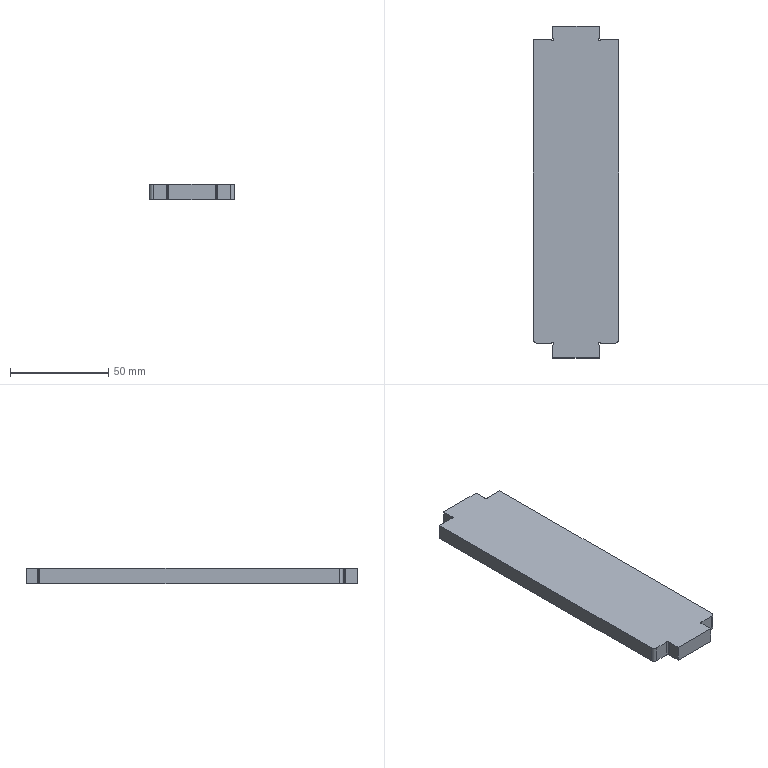Part | SolidWorks | features Fillet 2, FlatPattern 1, ICE 1, SMBaseFlange 1, SheetMetal 1 | 1 solid | 30 faces | box 43.5 x 169.3 x 8 mm | volume 56573 mm3 | cylinder 16 | plane 14 | commonest cylinder face diameters 2 x8 1 x6 4 x2
STEP:
#1=CARTESIAN_POINT('',(-156.793,-408.685,0.));
#2=VERTEX_POINT('',#1);
#3=CARTESIAN_POINT('',(-157.569,-409.102,0.));
#4=VERTEX_POINT('',#3);
#5=CARTESIAN_POINT('',(-157.069,-409.102,0.));
#6=DIRECTION('',(0.,0.,1.));
#7=DIRECTION('',(1.,0.,0.));
#8=AXIS2_PLACEMENT_3D('',#5,#6,#7);
#9=CIRCLE('',#8,0.5);
#10=EDGE_CURVE('',#2,#4,#9,.T.);
#11=ORIENTED_EDGE('',*,*,#10,.T.);
#12=CARTESIAN_POINT('',(-157.569,-409.102,-8.));
#13=VERTEX_POINT('',#12);
#14=CARTESIAN_POINT('',(-157.569,-409.102,-8.));
#15=DIRECTION('',(0.,0.,-1.));
#16=VECTOR('',#15,1000.);
#17=LINE('',#14,#16);
#18=EDGE_CURVE('',#4,#13,#17,.T.);
#19=ORIENTED_EDGE('',*,*,#18,.T.);
#20=CARTESIAN_POINT('',(-156.793,-408.685,-8.));
#21=VERTEX_POINT('',#20);
#22=CARTESIAN_POINT('',(-157.069,-409.102,-8.));
#23=DIRECTION('',(0.,0.,1.));
#24=DIRECTION('',(1.,0.,0.));
#25=AXIS2_PLACEMENT_3D('',#22,#23,#24);
#26=CIRCLE('',#25,0.5);
#27=EDGE_CURVE('',#21,#13,#26,.T.);
#28=ORIENTED_EDGE('',*,*,#27,.F.);
#29=CARTESIAN_POINT('',(-156.793,-408.685,-8.));
#30=DIRECTION('',(0.,0.,1.));
#31=VECTOR('',#30,1000.);
#32=LINE('',#29,#31);
#33=EDGE_CURVE('',#21,#2,#32,.T.);
#34=ORIENTED_EDGE('',*,*,#33,.T.);
#35=EDGE_LOOP('',(#11,#19,#28,#34));
#36=FACE_OUTER_BOUND('',#35,.T.);
#37=CARTESIAN_POINT('',(-157.069,-409.102,-8.));
#38=DIRECTION('',(0.,0.,-1.));
#39=DIRECTION('',(-1.,0.,0.));
#40=AXIS2_PLACEMENT_3D('',#37,#38,#39);
#41=CYLINDRICAL_SURFACE('',#40,0.5);
#42=ADVANCED_FACE('',(#36),#41,.F.);
#43=CARTESIAN_POINT('',(-157.486,-253.526,0.));
#44=VERTEX_POINT('',#43);
#45=CARTESIAN_POINT('',(-157.569,-253.802,0.));
#46=VERTEX_POINT('',#45);
#47=CARTESIAN_POINT('',(-157.069,-253.802,0.));
#48=DIRECTION('',(0.,0.,1.));
#49=DIRECTION('',(1.,0.,0.));
#50=AXIS2_PLACEMENT_3D('',#47,#48,#49);
#51=CIRCLE('',#50,0.5);
#52=EDGE_CURVE('',#44,#46,#51,.T.);
#53=ORIENTED_EDGE('',*,*,#52,.T.);
#54=CARTESIAN_POINT('',(-157.569,-253.802,-8.));
#55=VERTEX_POINT('',#54);
#56=CARTESIAN_POINT('',(-157.569,-253.802,-8.));
#57=DIRECTION('',(0.,0.,-1.));
#58=VECTOR('',#57,1000.);
#59=LINE('',#56,#58);
#60=EDGE_CURVE('',#46,#55,#59,.T.);
#61=ORIENTED_EDGE('',*,*,#60,.T.);
#62=CARTESIAN_POINT('',(-157.486,-253.526,-8.));
#63=VERTEX_POINT('',#62);
#64=CARTESIAN_POINT('',(-157.069,-253.802,-8.));
#65=DIRECTION('',(0.,0.,1.));
#66=DIRECTION('',(1.,0.,0.));
#67=AXIS2_PLACEMENT_3D('',#64,#65,#66);
#68=CIRCLE('',#67,0.5);
#69=EDGE_CURVE('',#63,#55,#68,.T.);
#70=ORIENTED_EDGE('',*,*,#69,.F.);
#71=CARTESIAN_POINT('',(-157.486,-253.526,-8.));
#72=DIRECTION('',(0.,0.,1.));
#73=VECTOR('',#72,1000.);
#74=LINE('',#71,#73);
#75=EDGE_CURVE('',#63,#44,#74,.T.);
#76=ORIENTED_EDGE('',*,*,#75,.T.);
#77=EDGE_LOOP('',(#53,#61,#70,#76));
#78=FACE_OUTER_BOUND('',#77,.T.);
#79=CARTESIAN_POINT('',(-157.069,-253.802,-8.));
#80=DIRECTION('',(0.,0.,-1.));
#81=DIRECTION('',(-1.,0.,0.));
#82=AXIS2_PLACEMENT_3D('',#79,#80,#81);
#83=CYLINDRICAL_SURFACE('',#82,0.5);
#84=ADVANCED_FACE('',(#78),#83,.F.);
#85=CARTESIAN_POINT('',(-188.819,-408.852,0.));
#86=VERTEX_POINT('',#85);
#87=CARTESIAN_POINT('',(-181.898,-408.852,0.));
#88=VERTEX_POINT('',#87);
#89=CARTESIAN_POINT('',(-180.819,-408.852,0.));
#90=DIRECTION('',(1.,0.,0.));
#91=VECTOR('',#90,1000.);
#92=LINE('',#89,#91);
#93=EDGE_CURVE('',#86,#88,#92,.T.);
#94=ORIENTED_EDGE('',*,*,#93,.F.);
#95=CARTESIAN_POINT('',(-188.819,-408.852,-8.));
#96=VERTEX_POINT('',#95);
#97=CARTESIAN_POINT('',(-188.819,-408.852,-8.));
#98=DIRECTION('',(0.,0.,-1.));
#99=VECTOR('',#98,1000.);
#100=LINE('',#97,#99);
#101=EDGE_CURVE('',#86,#96,#100,.T.);
#102=ORIENTED_EDGE('',*,*,#101,.T.);
#103=CARTESIAN_POINT('',(-181.898,-408.852,-8.));
#104=VERTEX_POINT('',#103);
#105=CARTESIAN_POINT('',(-180.819,-408.852,-8.));
#106=DIRECTION('',(1.,0.,0.));
#107=VECTOR('',#106,1000.);
#108=LINE('',#105,#107);
#109=EDGE_CURVE('',#96,#104,#108,.T.);
#110=ORIENTED_EDGE('',*,*,#109,.T.);
#111=CARTESIAN_POINT('',(-181.898,-408.852,-8.));
#112=DIRECTION('',(0.,0.,1.));
#113=VECTOR('',#112,1000.);
#114=LINE('',#111,#113);
#115=EDGE_CURVE('',#104,#88,#114,.T.);
#116=ORIENTED_EDGE('',*,*,#115,.T.);
#117=EDGE_LOOP('',(#94,#102,#110,#116));
#118=FACE_OUTER_BOUND('',#117,.T.);
#119=CARTESIAN_POINT('',(-180.819,-408.852,-8.));
#120=DIRECTION('',(0.,-1.,0.));
#121=DIRECTION('',(0.,0.,-1.));
#122=AXIS2_PLACEMENT_3D('',#119,#120,#121);
#123=PLANE('',#122);
#124=ADVANCED_FACE('',(#118),#123,.T.);
#125=CARTESIAN_POINT('',(-181.898,-254.052,0.));
#126=VERTEX_POINT('',#125);
#127=CARTESIAN_POINT('',(-190.819,-254.052,0.));
#128=VERTEX_POINT('',#127);
#129=CARTESIAN_POINT('',(-190.819,-254.052,0.));
#130=DIRECTION('',(-1.,0.,0.));
#131=VECTOR('',#130,1000.);
#132=LINE('',#129,#131);
#133=EDGE_CURVE('',#126,#128,#132,.T.);
#134=ORIENTED_EDGE('',*,*,#133,.F.);
#135=CARTESIAN_POINT('',(-181.898,-254.052,-8.));
#136=VERTEX_POINT('',#135);
#137=CARTESIAN_POINT('',(-181.898,-254.052,-8.));
#138=DIRECTION('',(0.,0.,-1.));
#139=VECTOR('',#138,1000.);
#140=LINE('',#137,#139);
#141=EDGE_CURVE('',#126,#136,#140,.T.);
#142=ORIENTED_EDGE('',*,*,#141,.T.);
#143=CARTESIAN_POINT('',(-190.819,-254.052,-8.));
#144=VERTEX_POINT('',#143);
#145=CARTESIAN_POINT('',(-190.819,-254.052,-8.));
#146=DIRECTION('',(-1.,0.,0.));
#147=VECTOR('',#146,1000.);
#148=LINE('',#145,#147);
#149=EDGE_CURVE('',#136,#144,#148,.T.);
#150=ORIENTED_EDGE('',*,*,#149,.T.);
#151=CARTESIAN_POINT('',(-190.819,-254.052,-8.));
#152=DIRECTION('',(0.,0.,1.));
#153=VECTOR('',#152,1000.);
#154=LINE('',#151,#153);
#155=EDGE_CURVE('',#144,#128,#154,.T.);
#156=ORIENTED_EDGE('',*,*,#155,.T.);
#157=EDGE_LOOP('',(#134,#142,#150,#156));
#158=FACE_OUTER_BOUND('',#157,.T.);
#159=CARTESIAN_POINT('',(-190.819,-254.052,-8.));
#160=DIRECTION('',(0.,1.,0.));
#161=DIRECTION('',(-1.,0.,0.));
#162=AXIS2_PLACEMENT_3D('',#159,#160,#161);
#163=PLANE('',#162);
#164=ADVANCED_FACE('',(#158),#163,.T.);
#165=CARTESIAN_POINT('',(-180.819,-247.052,-8.));
#166=VERTEX_POINT('',#165);
#167=CARTESIAN_POINT('',(-180.819,-252.973,-8.));
#168=VERTEX_POINT('',#167);
#169=CARTESIAN_POINT('',(-180.819,-247.052,-8.));
#170=DIRECTION('',(0.,-1.,0.));
#171=VECTOR('',#170,1000.);
#172=LINE('',#169,#171);
#173=EDGE_CURVE('',#166,#168,#172,.T.);
#174=ORIENTED_EDGE('',*,*,#173,.T.);
#175=CARTESIAN_POINT('',(-180.819,-252.973,0.));
#176=VERTEX_POINT('',#175);
#177=CARTESIAN_POINT('',(-180.819,-252.973,-8.));
#178=DIRECTION('',(0.,0.,1.));
#179=VECTOR('',#178,1000.);
#180=LINE('',#177,#179);
#181=EDGE_CURVE('',#168,#176,#180,.T.);
#182=ORIENTED_EDGE('',*,*,#181,.T.);
#183=CARTESIAN_POINT('',(-180.819,-247.052,0.));
#184=VERTEX_POINT('',#183);
#185=CARTESIAN_POINT('',(-180.819,-247.052,0.));
#186=DIRECTION('',(0.,-1.,0.));
#187=VECTOR('',#186,1000.);
#188=LINE('',#185,#187);
#189=EDGE_CURVE('',#184,#176,#188,.T.);
#190=ORIENTED_EDGE('',*,*,#189,.F.);
#191=CARTESIAN_POINT('',(-180.819,-247.052,-8.));
#192=DIRECTION('',(0.,0.,1.));
#193=VECTOR('',#192,1000.);
#194=LINE('',#191,#193);
#195=EDGE_CURVE('',#166,#184,#194,.T.);
#196=ORIENTED_EDGE('',*,*,#195,.F.);
#197=EDGE_LOOP('',(#174,#182,#190,#196));
#198=FACE_OUTER_BOUND('',#197,.T.);
#199=CARTESIAN_POINT('',(-180.819,-247.052,-8.));
#200=DIRECTION('',(-1.,0.,0.));
#201=DIRECTION('',(0.,-1.,0.));
#202=AXIS2_PLACEMENT_3D('',#199,#200,#201);
#203=PLANE('',#202);
#204=ADVANCED_FACE('',(#198),#203,.T.);
#205=CARTESIAN_POINT('',(-157.319,-252.973,0.));
#206=VERTEX_POINT('',#205);
#207=CARTESIAN_POINT('',(-157.319,-247.052,0.));
#208=VERTEX_POINT('',#207);
#209=CARTESIAN_POINT('',(-157.319,-254.052,0.));
#210=DIRECTION('',(0.,1.,0.));
#211=VECTOR('',#210,1000.);
#212=LINE('',#209,#211);
#213=EDGE_CURVE('',#206,#208,#212,.T.);
#214=ORIENTED_EDGE('',*,*,#213,.F.);
#215=CARTESIAN_POINT('',(-157.319,-252.973,-8.));
#216=VERTEX_POINT('',#215);
#217=CARTESIAN_POINT('',(-157.319,-252.973,-8.));
#218=DIRECTION('',(0.,0.,-1.));
#219=VECTOR('',#218,1000.);
#220=LINE('',#217,#219);
#221=EDGE_CURVE('',#206,#216,#220,.T.);
#222=ORIENTED_EDGE('',*,*,#221,.T.);
#223=CARTESIAN_POINT('',(-157.319,-247.052,-8.));
#224=VERTEX_POINT('',#223);
#225=CARTESIAN_POINT('',(-157.319,-254.052,-8.));
#226=DIRECTION('',(0.,1.,0.));
#227=VECTOR('',#226,1000.);
#228=LINE('',#225,#227);
#229=EDGE_CURVE('',#216,#224,#228,.T.);
#230=ORIENTED_EDGE('',*,*,#229,.T.);
#231=CARTESIAN_POINT('',(-157.319,-247.052,-8.));
#232=DIRECTION('',(0.,0.,1.));
#233=VECTOR('',#232,1000.);
#234=LINE('',#231,#233);
#235=EDGE_CURVE('',#224,#208,#234,.T.);
#236=ORIENTED_EDGE('',*,*,#235,.T.);
#237=EDGE_LOOP('',(#214,#222,#230,#236));
#238=FACE_OUTER_BOUND('',#237,.T.);
#239=CARTESIAN_POINT('',(-157.319,-254.052,-8.));
#240=DIRECTION('',(1.,0.,0.));
#241=DIRECTION('',(0.,1.,0.));
#242=AXIS2_PLACEMENT_3D('',#239,#240,#241);
#243=PLANE('',#242);
#244=ADVANCED_FACE('',(#238),#243,.T.);
#245=CARTESIAN_POINT('',(-147.319,-254.052,-8.));
#246=VERTEX_POINT('',#245);
#247=CARTESIAN_POINT('',(-156.24,-254.052,-8.));
#248=VERTEX_POINT('',#247);
#249=CARTESIAN_POINT('',(-157.319,-254.052,-8.));
#250=DIRECTION('',(-1.,0.,0.));
#251=VECTOR('',#250,1000.);
#252=LINE('',#249,#251);
#253=EDGE_CURVE('',#246,#248,#252,.T.);
#254=ORIENTED_EDGE('',*,*,#253,.T.);
#255=CARTESIAN_POINT('',(-156.24,-254.052,0.));
#256=VERTEX_POINT('',#255);
#257=CARTESIAN_POINT('',(-156.24,-254.052,-8.));
#258=DIRECTION('',(0.,0.,1.));
#259=VECTOR('',#258,1000.);
#260=LINE('',#257,#259);
#261=EDGE_CURVE('',#248,#256,#260,.T.);
#262=ORIENTED_EDGE('',*,*,#261,.T.);
#263=CARTESIAN_POINT('',(-147.319,-254.052,0.));
#264=VERTEX_POINT('',#263);
#265=CARTESIAN_POINT('',(-157.319,-254.052,0.));
#266=DIRECTION('',(-1.,0.,0.));
#267=VECTOR('',#266,1000.);
#268=LINE('',#265,#267);
#269=EDGE_CURVE('',#264,#256,#268,.T.);
#270=ORIENTED_EDGE('',*,*,#269,.F.);
#271=CARTESIAN_POINT('',(-147.319,-254.052,-8.));
#272=DIRECTION('',(0.,0.,1.));
#273=VECTOR('',#272,1000.);
#274=LINE('',#271,#273);
#275=EDGE_CURVE('',#246,#264,#274,.T.);
#276=ORIENTED_EDGE('',*,*,#275,.F.);
#277=EDGE_LOOP('',(#254,#262,#270,#276));
#278=FACE_OUTER_BOUND('',#277,.T.);
#279=CARTESIAN_POINT('',(-157.319,-254.052,-8.));
#280=DIRECTION('',(0.,1.,0.));
#281=DIRECTION('',(-1.,0.,0.));
#282=AXIS2_PLACEMENT_3D('',#279,#280,#281);
#283=PLANE('',#282);
#284=ADVANCED_FACE('',(#278),#283,.T.);
#285=CARTESIAN_POINT('',(-156.24,-408.852,-8.));
#286=VERTEX_POINT('',#285);
#287=CARTESIAN_POINT('',(-149.319,-408.852,-8.));
#288=VERTEX_POINT('',#287);
#289=CARTESIAN_POINT('',(-147.319,-408.852,-8.));
#290=DIRECTION('',(1.,0.,0.));
#291=VECTOR('',#290,1000.);
#292=LINE('',#289,#291);
#293=EDGE_CURVE('',#286,#288,#292,.T.);
#294=ORIENTED_EDGE('',*,*,#293,.T.);
#295=CARTESIAN_POINT('',(-149.319,-408.852,0.));
#296=VERTEX_POINT('',#295);
#297=CARTESIAN_POINT('',(-149.319,-408.852,-8.));
#298=DIRECTION('',(0.,0.,1.));
#299=VECTOR('',#298,1000.);
#300=LINE('',#297,#299);
#301=EDGE_CURVE('',#288,#296,#300,.T.);
#302=ORIENTED_EDGE('',*,*,#301,.T.);
#303=CARTESIAN_POINT('',(-156.24,-408.852,0.));
#304=VERTEX_POINT('',#303);
#305=CARTESIAN_POINT('',(-147.319,-408.852,0.));
#306=DIRECTION('',(1.,0.,0.));
#307=VECTOR('',#306,1000.);
#308=LINE('',#305,#307);
#309=EDGE_CURVE('',#304,#296,#308,.T.);
#310=ORIENTED_EDGE('',*,*,#309,.F.);
#311=CARTESIAN_POINT('',(-156.24,-408.852,-8.));
#312=DIRECTION('',(0.,0.,-1.));
#313=VECTOR('',#312,1000.);
#314=LINE('',#311,#313);
#315=EDGE_CURVE('',#304,#286,#314,.T.);
#316=ORIENTED_EDGE('',*,*,#315,.T.);
#317=EDGE_LOOP('',(#294,#302,#310,#316));
#318=FACE_OUTER_BOUND('',#317,.T.);
#319=CARTESIAN_POINT('',(-147.319,-408.852,-8.));
#320=DIRECTION('',(0.,-1.,0.));
#321=DIRECTION('',(1.,0.,0.));
#322=AXIS2_PLACEMENT_3D('',#319,#320,#321);
#323=PLANE('',#322);
#324=ADVANCED_FACE('',(#318),#323,.T.);
#325=CARTESIAN_POINT('',(-157.319,-416.352,-8.));
#326=VERTEX_POINT('',#325);
#327=CARTESIAN_POINT('',(-157.319,-409.931,-8.));
#328=VERTEX_POINT('',#327);
#329=CARTESIAN_POINT('',(-157.319,-408.852,-8.));
#330=DIRECTION('',(0.,1.,0.));
#331=VECTOR('',#330,1000.);
#332=LINE('',#329,#331);
#333=EDGE_CURVE('',#326,#328,#332,.T.);
#334=ORIENTED_EDGE('',*,*,#333,.T.);
#335=CARTESIAN_POINT('',(-157.319,-409.931,0.));
#336=VERTEX_POINT('',#335);
#337=CARTESIAN_POINT('',(-157.319,-409.931,-8.));
#338=DIRECTION('',(0.,0.,1.));
#339=VECTOR('',#338,1000.);
#340=LINE('',#337,#339);
#341=EDGE_CURVE('',#328,#336,#340,.T.);
#342=ORIENTED_EDGE('',*,*,#341,.T.);
#343=CARTESIAN_POINT('',(-157.319,-416.352,0.));
#344=VERTEX_POINT('',#343);
#345=CARTESIAN_POINT('',(-157.319,-408.852,0.));
#346=DIRECTION('',(0.,1.,0.));
#347=VECTOR('',#346,1000.);
#348=LINE('',#345,#347);
#349=EDGE_CURVE('',#344,#336,#348,.T.);
#350=ORIENTED_EDGE('',*,*,#349,.F.);
#351=CARTESIAN_POINT('',(-157.319,-416.352,-8.));
#352=DIRECTION('',(0.,0.,1.));
#353=VECTOR('',#352,1000.);
#354=LINE('',#351,#353);
#355=EDGE_CURVE('',#326,#344,#354,.T.);
#356=ORIENTED_EDGE('',*,*,#355,.F.);
#357=EDGE_LOOP('',(#334,#342,#350,#356));
#358=FACE_OUTER_BOUND('',#357,.T.);
#359=CARTESIAN_POINT('',(-157.319,-408.852,-8.));
#360=DIRECTION('',(1.,0.,0.));
#361=DIRECTION('',(0.,0.,-1.));
#362=AXIS2_PLACEMENT_3D('',#359,#360,#361);
#363=PLANE('',#362);
#364=ADVANCED_FACE('',(#358),#363,.T.);
#365=CARTESIAN_POINT('',(-180.819,-409.931,0.));
#366=VERTEX_POINT('',#365);
#367=CARTESIAN_POINT('',(-180.819,-416.352,0.));
#368=VERTEX_POINT('',#367);
#369=CARTESIAN_POINT('',(-180.819,-416.352,0.));
#370=DIRECTION('',(0.,-1.,0.));
#371=VECTOR('',#370,1000.);
#372=LINE('',#369,#371);
#373=EDGE_CURVE('',#366,#368,#372,.T.);
#374=ORIENTED_EDGE('',*,*,#373,.F.);
#375=CARTESIAN_POINT('',(-180.819,-409.931,-8.));
#376=VERTEX_POINT('',#375);
#377=CARTESIAN_POINT('',(-180.819,-409.931,-8.));
#378=DIRECTION('',(0.,0.,-1.));
#379=VECTOR('',#378,1000.);
#380=LINE('',#377,#379);
#381=EDGE_CURVE('',#366,#376,#380,.T.);
#382=ORIENTED_EDGE('',*,*,#381,.T.);
#383=CARTESIAN_POINT('',(-180.819,-416.352,-8.));
#384=VERTEX_POINT('',#383);
#385=CARTESIAN_POINT('',(-180.819,-416.352,-8.));
#386=DIRECTION('',(0.,-1.,0.));
#387=VECTOR('',#386,1000.);
#388=LINE('',#385,#387);
#389=EDGE_CURVE('',#376,#384,#388,.T.);
#390=ORIENTED_EDGE('',*,*,#389,.T.);
#391=CARTESIAN_POINT('',(-180.819,-416.352,-8.));
#392=DIRECTION('',(0.,0.,1.));
#393=VECTOR('',#392,1000.);
#394=LINE('',#391,#393);
#395=EDGE_CURVE('',#384,#368,#394,.T.);
#396=ORIENTED_EDGE('',*,*,#395,.T.);
#397=EDGE_LOOP('',(#374,#382,#390,#396));
#398=FACE_OUTER_BOUND('',#397,.T.);
#399=CARTESIAN_POINT('',(-180.819,-416.352,-8.));
#400=DIRECTION('',(-1.,0.,0.));
#401=DIRECTION('',(0.,-1.,0.));
#402=AXIS2_PLACEMENT_3D('',#399,#400,#401);
#403=PLANE('',#402);
#404=ADVANCED_FACE('',(#398),#403,.T.);
#405=ORIENTED_EDGE('',*,*,#109,.F.);
#406=CARTESIAN_POINT('',(-190.819,-406.852,-8.));
#407=VERTEX_POINT('',#406);
#408=CARTESIAN_POINT('',(-188.819,-406.852,-8.));
#409=DIRECTION('',(0.,0.,-1.));
#410=DIRECTION('',(-1.,0.,0.));
#411=AXIS2_PLACEMENT_3D('',#408,#409,#410);
#412=CIRCLE('',#411,2.);
#413=EDGE_CURVE('',#96,#407,#412,.T.);
#414=ORIENTED_EDGE('',*,*,#413,.T.);
#415=CARTESIAN_POINT('',(-190.819,-408.852,-8.));
#416=DIRECTION('',(0.,-1.,0.));
#417=VECTOR('',#416,1000.);
#418=LINE('',#415,#417);
#419=EDGE_CURVE('',#144,#407,#418,.T.);
#420=ORIENTED_EDGE('',*,*,#419,.F.);
#421=ORIENTED_EDGE('',*,*,#149,.F.);
#422=CARTESIAN_POINT('',(-181.346,-254.219,-8.));
#423=VERTEX_POINT('',#422);
#424=CARTESIAN_POINT('',(-181.898,-255.052,-8.));
#425=DIRECTION('',(0.,0.,-1.));
#426=DIRECTION('',(-1.,0.,0.));
#427=AXIS2_PLACEMENT_3D('',#424,#425,#426);
#428=CIRCLE('',#427,1.);
#429=EDGE_CURVE('',#136,#423,#428,.T.);
#430=ORIENTED_EDGE('',*,*,#429,.T.);
#431=CARTESIAN_POINT('',(-180.653,-253.526,-8.));
#432=VERTEX_POINT('',#431);
#433=CARTESIAN_POINT('',(-181.069,-253.802,-8.));
#434=DIRECTION('',(0.,0.,1.));
#435=DIRECTION('',(1.,0.,0.));
#436=AXIS2_PLACEMENT_3D('',#433,#434,#435);
#437=CIRCLE('',#436,0.5);
#438=EDGE_CURVE('',#423,#432,#437,.T.);
#439=ORIENTED_EDGE('',*,*,#438,.T.);
#440=CARTESIAN_POINT('',(-179.819,-252.973,-8.));
#441=DIRECTION('',(0.,0.,-1.));
#442=DIRECTION('',(-1.,0.,0.));
#443=AXIS2_PLACEMENT_3D('',#440,#441,#442);
#444=CIRCLE('',#443,1.);
#445=EDGE_CURVE('',#432,#168,#444,.T.);
#446=ORIENTED_EDGE('',*,*,#445,.T.);
#447=ORIENTED_EDGE('',*,*,#173,.F.);
#448=CARTESIAN_POINT('',(-157.319,-247.052,-8.));
#449=DIRECTION('',(-1.,0.,0.));
#450=VECTOR('',#449,1000.);
#451=LINE('',#448,#450);
#452=EDGE_CURVE('',#224,#166,#451,.T.);
#453=ORIENTED_EDGE('',*,*,#452,.F.);
#454=ORIENTED_EDGE('',*,*,#229,.F.);
#455=CARTESIAN_POINT('',(-158.319,-252.973,-8.));
#456=DIRECTION('',(0.,0.,-1.));
#457=DIRECTION('',(-1.,0.,0.));
#458=AXIS2_PLACEMENT_3D('',#455,#456,#457);
#459=CIRCLE('',#458,1.);
#460=EDGE_CURVE('',#216,#63,#459,.T.);
#461=ORIENTED_EDGE('',*,*,#460,.T.);
#462=ORIENTED_EDGE('',*,*,#69,.T.);
#463=CARTESIAN_POINT('',(-156.793,-254.219,-8.));
#464=VERTEX_POINT('',#463);
#465=CARTESIAN_POINT('',(-157.069,-253.802,-8.));
#466=DIRECTION('',(0.,0.,1.));
#467=DIRECTION('',(1.,0.,0.));
#468=AXIS2_PLACEMENT_3D('',#465,#466,#467);
#469=CIRCLE('',#468,0.5);
#470=EDGE_CURVE('',#55,#464,#469,.T.);
#471=ORIENTED_EDGE('',*,*,#470,.T.);
#472=CARTESIAN_POINT('',(-156.24,-255.052,-8.));
#473=DIRECTION('',(0.,0.,-1.));
#474=DIRECTION('',(-1.,0.,0.));
#475=AXIS2_PLACEMENT_3D('',#472,#473,#474);
#476=CIRCLE('',#475,1.);
#477=EDGE_CURVE('',#464,#248,#476,.T.);
#478=ORIENTED_EDGE('',*,*,#477,.T.);
#479=ORIENTED_EDGE('',*,*,#253,.F.);
#480=CARTESIAN_POINT('',(-147.319,-406.852,-8.));
#481=VERTEX_POINT('',#480);
#482=CARTESIAN_POINT('',(-147.319,-254.052,-8.));
#483=DIRECTION('',(0.,1.,0.));
#484=VECTOR('',#483,1000.);
#485=LINE('',#482,#484);
#486=EDGE_CURVE('',#481,#246,#485,.T.);
#487=ORIENTED_EDGE('',*,*,#486,.F.);
#488=CARTESIAN_POINT('',(-149.319,-406.852,-8.));
#489=DIRECTION('',(0.,0.,-1.));
#490=DIRECTION('',(-1.,0.,0.));
#491=AXIS2_PLACEMENT_3D('',#488,#489,#490);
#492=CIRCLE('',#491,2.);
#493=EDGE_CURVE('',#481,#288,#492,.T.);
#494=ORIENTED_EDGE('',*,*,#493,.T.);
#495=ORIENTED_EDGE('',*,*,#293,.F.);
#496=CARTESIAN_POINT('',(-156.24,-407.852,-8.));
#497=DIRECTION('',(0.,0.,-1.));
#498=DIRECTION('',(-1.,0.,0.));
#499=AXIS2_PLACEMENT_3D('',#496,#497,#498);
#500=CIRCLE('',#499,1.);
#501=EDGE_CURVE('',#286,#21,#500,.T.);
#502=ORIENTED_EDGE('',*,*,#501,.T.);
#503=ORIENTED_EDGE('',*,*,#27,.T.);
#504=CARTESIAN_POINT('',(-157.486,-409.378,-8.));
#505=VERTEX_POINT('',#504);
#506=CARTESIAN_POINT('',(-157.069,-409.102,-8.));
#507=DIRECTION('',(0.,0.,1.));
#508=DIRECTION('',(1.,0.,0.));
#509=AXIS2_PLACEMENT_3D('',#506,#507,#508);
#510=CIRCLE('',#509,0.5);
#511=EDGE_CURVE('',#13,#505,#510,.T.);
#512=ORIENTED_EDGE('',*,*,#511,.T.);
#513=CARTESIAN_POINT('',(-158.319,-409.931,-8.));
#514=DIRECTION('',(0.,0.,-1.));
#515=DIRECTION('',(-1.,0.,0.));
#516=AXIS2_PLACEMENT_3D('',#513,#514,#515);
#517=CIRCLE('',#516,1.);
#518=EDGE_CURVE('',#505,#328,#517,.T.);
#519=ORIENTED_EDGE('',*,*,#518,.T.);
#520=ORIENTED_EDGE('',*,*,#333,.F.);
#521=CARTESIAN_POINT('',(-157.319,-416.352,-8.));
#522=DIRECTION('',(1.,0.,0.));
#523=VECTOR('',#522,1000.);
#524=LINE('',#521,#523);
#525=EDGE_CURVE('',#384,#326,#524,.T.);
#526=ORIENTED_EDGE('',*,*,#525,.F.);
#527=ORIENTED_EDGE('',*,*,#389,.F.);
#528=CARTESIAN_POINT('',(-180.653,-409.378,-8.));
#529=VERTEX_POINT('',#528);
#530=CARTESIAN_POINT('',(-179.819,-409.931,-8.));
#531=DIRECTION('',(0.,0.,-1.));
#532=DIRECTION('',(-1.,0.,0.));
#533=AXIS2_PLACEMENT_3D('',#530,#531,#532);
#534=CIRCLE('',#533,1.);
#535=EDGE_CURVE('',#376,#529,#534,.T.);
#536=ORIENTED_EDGE('',*,*,#535,.T.);
#537=CARTESIAN_POINT('',(-181.346,-408.685,-8.));
#538=VERTEX_POINT('',#537);
#539=CARTESIAN_POINT('',(-181.069,-409.102,-8.));
#540=DIRECTION('',(0.,0.,-1.));
#541=DIRECTION('',(-1.,0.,0.));
#542=AXIS2_PLACEMENT_3D('',#539,#540,#541);
#543=CIRCLE('',#542,0.5);
#544=EDGE_CURVE('',#538,#529,#543,.T.);
#545=ORIENTED_EDGE('',*,*,#544,.F.);
#546=CARTESIAN_POINT('',(-181.898,-407.852,-8.));
#547=DIRECTION('',(0.,0.,-1.));
#548=DIRECTION('',(-1.,0.,0.));
#549=AXIS2_PLACEMENT_3D('',#546,#547,#548);
#550=CIRCLE('',#549,1.);
#551=EDGE_CURVE('',#538,#104,#550,.T.);
#552=ORIENTED_EDGE('',*,*,#551,.T.);
#553=EDGE_LOOP('',(#405,#414,#420,#421,#430,#439,#446,#447,#453,#454,#461,#462,#471,#478,#479,#487,#494,#495,#502,#503,#512,#519,#520,#526,#527,#536,#545,#552));
#554=FACE_OUTER_BOUND('',#553,.T.);
#555=CARTESIAN_POINT('',(0.,0.,-8.));
#556=DIRECTION('',(0.,0.,-1.));
#557=DIRECTION('',(-1.,0.,0.));
#558=AXIS2_PLACEMENT_3D('',#555,#556,#557);
#559=PLANE('',#558);
#560=ADVANCED_FACE('',(#554),#559,.T.);
#561=CARTESIAN_POINT('',(-190.819,-406.852,0.));
#562=VERTEX_POINT('',#561);
#563=CARTESIAN_POINT('',(-190.819,-408.852,0.));
#564=DIRECTION('',(0.,-1.,0.));
#565=VECTOR('',#564,1000.);
#566=LINE('',#563,#565);
#567=EDGE_CURVE('',#128,#562,#566,.T.);
#568=ORIENTED_EDGE('',*,*,#567,.T.);
#569=CARTESIAN_POINT('',(-188.819,-406.852,0.));
#570=DIRECTION('',(0.,0.,1.));
#571=DIRECTION('',(-1.,0.,0.));
#572=AXIS2_PLACEMENT_3D('',#569,#570,#571);
#573=CIRCLE('',#572,2.);
#574=EDGE_CURVE('',#562,#86,#573,.T.);
#575=ORIENTED_EDGE('',*,*,#574,.T.);
#576=ORIENTED_EDGE('',*,*,#93,.T.);
#577=CARTESIAN_POINT('',(-181.346,-408.685,0.));
#578=VERTEX_POINT('',#577);
#579=CARTESIAN_POINT('',(-181.898,-407.852,0.));
#580=DIRECTION('',(0.,0.,1.));
#581=DIRECTION('',(-1.,0.,0.));
#582=AXIS2_PLACEMENT_3D('',#579,#580,#581);
#583=CIRCLE('',#582,1.);
#584=EDGE_CURVE('',#88,#578,#583,.T.);
#585=ORIENTED_EDGE('',*,*,#584,.T.);
#586=CARTESIAN_POINT('',(-180.653,-409.378,0.));
#587=VERTEX_POINT('',#586);
#588=CARTESIAN_POINT('',(-181.069,-409.102,0.));
#589=DIRECTION('',(0.,0.,-1.));
#590=DIRECTION('',(-1.,0.,0.));
#591=AXIS2_PLACEMENT_3D('',#588,#589,#590);
#592=CIRCLE('',#591,0.5);
#593=EDGE_CURVE('',#578,#587,#592,.T.);
#594=ORIENTED_EDGE('',*,*,#593,.T.);
#595=CARTESIAN_POINT('',(-179.819,-409.931,0.));
#596=DIRECTION('',(0.,0.,1.));
#597=DIRECTION('',(-1.,0.,0.));
#598=AXIS2_PLACEMENT_3D('',#595,#596,#597);
#599=CIRCLE('',#598,1.);
#600=EDGE_CURVE('',#587,#366,#599,.T.);
#601=ORIENTED_EDGE('',*,*,#600,.T.);
#602=ORIENTED_EDGE('',*,*,#373,.T.);
#603=CARTESIAN_POINT('',(-157.319,-416.352,0.));
#604=DIRECTION('',(1.,0.,0.));
#605=VECTOR('',#604,1000.);
#606=LINE('',#603,#605);
#607=EDGE_CURVE('',#368,#344,#606,.T.);
#608=ORIENTED_EDGE('',*,*,#607,.T.);
#609=ORIENTED_EDGE('',*,*,#349,.T.);
#610=CARTESIAN_POINT('',(-157.486,-409.378,0.));
#611=VERTEX_POINT('',#610);
#612=CARTESIAN_POINT('',(-158.319,-409.931,0.));
#613=DIRECTION('',(0.,0.,1.));
#614=DIRECTION('',(-1.,0.,0.));
#615=AXIS2_PLACEMENT_3D('',#612,#613,#614);
#616=CIRCLE('',#615,1.);
#617=EDGE_CURVE('',#336,#611,#616,.T.);
#618=ORIENTED_EDGE('',*,*,#617,.T.);
#619=CARTESIAN_POINT('',(-157.069,-409.102,0.));
#620=DIRECTION('',(0.,0.,1.));
#621=DIRECTION('',(1.,0.,0.));
#622=AXIS2_PLACEMENT_3D('',#619,#620,#621);
#623=CIRCLE('',#622,0.5);
#624=EDGE_CURVE('',#4,#611,#623,.T.);
#625=ORIENTED_EDGE('',*,*,#624,.F.);
#626=ORIENTED_EDGE('',*,*,#10,.F.);
#627=CARTESIAN_POINT('',(-156.24,-407.852,0.));
#628=DIRECTION('',(0.,0.,1.));
#629=DIRECTION('',(-1.,0.,0.));
#630=AXIS2_PLACEMENT_3D('',#627,#628,#629);
#631=CIRCLE('',#630,1.);
#632=EDGE_CURVE('',#2,#304,#631,.T.);
#633=ORIENTED_EDGE('',*,*,#632,.T.);
#634=ORIENTED_EDGE('',*,*,#309,.T.);
#635=CARTESIAN_POINT('',(-147.319,-406.852,0.));
#636=VERTEX_POINT('',#635);
#637=CARTESIAN_POINT('',(-149.319,-406.852,0.));
#638=DIRECTION('',(0.,0.,1.));
#639=DIRECTION('',(-1.,0.,0.));
#640=AXIS2_PLACEMENT_3D('',#637,#638,#639);
#641=CIRCLE('',#640,2.);
#642=EDGE_CURVE('',#296,#636,#641,.T.);
#643=ORIENTED_EDGE('',*,*,#642,.T.);
#644=CARTESIAN_POINT('',(-147.319,-254.052,0.));
#645=DIRECTION('',(0.,1.,0.));
#646=VECTOR('',#645,1000.);
#647=LINE('',#644,#646);
#648=EDGE_CURVE('',#636,#264,#647,.T.);
#649=ORIENTED_EDGE('',*,*,#648,.T.);
#650=ORIENTED_EDGE('',*,*,#269,.T.);
#651=CARTESIAN_POINT('',(-156.793,-254.219,0.));
#652=VERTEX_POINT('',#651);
#653=CARTESIAN_POINT('',(-156.24,-255.052,0.));
#654=DIRECTION('',(0.,0.,1.));
#655=DIRECTION('',(-1.,0.,0.));
#656=AXIS2_PLACEMENT_3D('',#653,#654,#655);
#657=CIRCLE('',#656,1.);
#658=EDGE_CURVE('',#256,#652,#657,.T.);
#659=ORIENTED_EDGE('',*,*,#658,.T.);
#660=CARTESIAN_POINT('',(-157.069,-253.802,0.));
#661=DIRECTION('',(0.,0.,1.));
#662=DIRECTION('',(1.,0.,0.));
#663=AXIS2_PLACEMENT_3D('',#660,#661,#662);
#664=CIRCLE('',#663,0.5);
#665=EDGE_CURVE('',#46,#652,#664,.T.);
#666=ORIENTED_EDGE('',*,*,#665,.F.);
#667=ORIENTED_EDGE('',*,*,#52,.F.);
#668=CARTESIAN_POINT('',(-158.319,-252.973,0.));
#669=DIRECTION('',(0.,0.,1.));
#670=DIRECTION('',(-1.,0.,0.));
#671=AXIS2_PLACEMENT_3D('',#668,#669,#670);
#672=CIRCLE('',#671,1.);
#673=EDGE_CURVE('',#44,#206,#672,.T.);
#674=ORIENTED_EDGE('',*,*,#673,.T.);
#675=ORIENTED_EDGE('',*,*,#213,.T.);
#676=CARTESIAN_POINT('',(-157.319,-247.052,0.));
#677=DIRECTION('',(-1.,0.,0.));
#678=VECTOR('',#677,1000.);
#679=LINE('',#676,#678);
#680=EDGE_CURVE('',#208,#184,#679,.T.);
#681=ORIENTED_EDGE('',*,*,#680,.T.);
#682=ORIENTED_EDGE('',*,*,#189,.T.);
#683=CARTESIAN_POINT('',(-180.653,-253.526,0.));
#684=VERTEX_POINT('',#683);
#685=CARTESIAN_POINT('',(-179.819,-252.973,0.));
#686=DIRECTION('',(0.,0.,1.));
#687=DIRECTION('',(-1.,0.,0.));
#688=AXIS2_PLACEMENT_3D('',#685,#686,#687);
#689=CIRCLE('',#688,1.);
#690=EDGE_CURVE('',#176,#684,#689,.T.);
#691=ORIENTED_EDGE('',*,*,#690,.T.);
#692=CARTESIAN_POINT('',(-181.346,-254.219,0.));
#693=VERTEX_POINT('',#692);
#694=CARTESIAN_POINT('',(-181.069,-253.802,0.));
#695=DIRECTION('',(0.,0.,1.));
#696=DIRECTION('',(1.,0.,0.));
#697=AXIS2_PLACEMENT_3D('',#694,#695,#696);
#698=CIRCLE('',#697,0.5);
#699=EDGE_CURVE('',#693,#684,#698,.T.);
#700=ORIENTED_EDGE('',*,*,#699,.F.);
#701=CARTESIAN_POINT('',(-181.898,-255.052,0.));
#702=DIRECTION('',(0.,0.,1.));
#703=DIRECTION('',(-1.,0.,0.));
#704=AXIS2_PLACEMENT_3D('',#701,#702,#703);
#705=CIRCLE('',#704,1.);
#706=EDGE_CURVE('',#693,#126,#705,.T.);
#707=ORIENTED_EDGE('',*,*,#706,.T.);
#708=ORIENTED_EDGE('',*,*,#133,.T.);
#709=EDGE_LOOP('',(#568,#575,#576,#585,#594,#601,#602,#608,#609,#618,#625,#626,#633,#634,#643,#649,#650,#659,#666,#667,#674,#675,#681,#682,#691,#700,#707,#708));
#710=FACE_OUTER_BOUND('',#709,.T.);
#711=CARTESIAN_POINT('',(0.,0.,0.));
#712=DIRECTION('',(0.,0.,-1.));
#713=DIRECTION('',(-1.,0.,0.));
#714=AXIS2_PLACEMENT_3D('',#711,#712,#713);
#715=PLANE('',#714);
#716=ADVANCED_FACE('',(#710),#715,.F.);
#717=ORIENTED_EDGE('',*,*,#419,.T.);
#718=CARTESIAN_POINT('',(-190.819,-406.852,-8.));
#719=DIRECTION('',(0.,0.,1.));
#720=VECTOR('',#719,1000.);
#721=LINE('',#718,#720);
#722=EDGE_CURVE('',#407,#562,#721,.T.);
#723=ORIENTED_EDGE('',*,*,#722,.T.);
#724=ORIENTED_EDGE('',*,*,#567,.F.);
#725=ORIENTED_EDGE('',*,*,#155,.F.);
#726=EDGE_LOOP('',(#717,#723,#724,#725));
#727=FACE_OUTER_BOUND('',#726,.T.);
#728=CARTESIAN_POINT('',(-190.819,-408.852,-8.));
#729=DIRECTION('',(-1.,0.,0.));
#730=DIRECTION('',(0.,-1.,0.));
#731=AXIS2_PLACEMENT_3D('',#728,#729,#730);
#732=PLANE('',#731);
#733=ADVANCED_FACE('',(#727),#732,.T.);
#734=ORIENTED_EDGE('',*,*,#680,.F.);
#735=ORIENTED_EDGE('',*,*,#235,.F.);
#736=ORIENTED_EDGE('',*,*,#452,.T.);
#737=ORIENTED_EDGE('',*,*,#195,.T.);
#738=EDGE_LOOP('',(#734,#735,#736,#737));
#739=FACE_OUTER_BOUND('',#738,.T.);
#740=CARTESIAN_POINT('',(-157.319,-247.052,-8.));
#741=DIRECTION('',(0.,1.,0.));
#742=DIRECTION('',(-1.,0.,0.));
#743=AXIS2_PLACEMENT_3D('',#740,#741,#742);
#744=PLANE('',#743);
#745=ADVANCED_FACE('',(#739),#744,.T.);
#746=ORIENTED_EDGE('',*,*,#648,.F.);
#747=CARTESIAN_POINT('',(-147.319,-406.852,-8.));
#748=DIRECTION('',(0.,0.,-1.));
#749=VECTOR('',#748,1000.);
#750=LINE('',#747,#749);
#751=EDGE_CURVE('',#636,#481,#750,.T.);
#752=ORIENTED_EDGE('',*,*,#751,.T.);
#753=ORIENTED_EDGE('',*,*,#486,.T.);
#754=ORIENTED_EDGE('',*,*,#275,.T.);
#755=EDGE_LOOP('',(#746,#752,#753,#754));
#756=FACE_OUTER_BOUND('',#755,.T.);
#757=CARTESIAN_POINT('',(-147.319,-254.052,-8.));
#758=DIRECTION('',(1.,0.,0.));
#759=DIRECTION('',(0.,1.,0.));
#760=AXIS2_PLACEMENT_3D('',#757,#758,#759);
#761=PLANE('',#760);
#762=ADVANCED_FACE('',(#756),#761,.T.);
#763=ORIENTED_EDGE('',*,*,#607,.F.);
#764=ORIENTED_EDGE('',*,*,#395,.F.);
#765=ORIENTED_EDGE('',*,*,#525,.T.);
#766=ORIENTED_EDGE('',*,*,#355,.T.);
#767=EDGE_LOOP('',(#763,#764,#765,#766));
#768=FACE_OUTER_BOUND('',#767,.T.);
#769=CARTESIAN_POINT('',(-157.319,-416.352,-8.));
#770=DIRECTION('',(0.,-1.,0.));
#771=DIRECTION('',(0.,0.,-1.));
#772=AXIS2_PLACEMENT_3D('',#769,#770,#771);
#773=PLANE('',#772);
#774=ADVANCED_FACE('',(#768),#773,.T.);
#775=ORIENTED_EDGE('',*,*,#544,.T.);
#776=CARTESIAN_POINT('',(-180.653,-409.378,0.));
#777=DIRECTION('',(0.,0.,1.));
#778=VECTOR('',#777,1000.);
#779=LINE('',#776,#778);
#780=EDGE_CURVE('',#529,#587,#779,.T.);
#781=ORIENTED_EDGE('',*,*,#780,.T.);
#782=ORIENTED_EDGE('',*,*,#593,.F.);
#783=CARTESIAN_POINT('',(-181.346,-408.685,0.));
#784=DIRECTION('',(0.,0.,-1.));
#785=VECTOR('',#784,1000.);
#786=LINE('',#783,#785);
#787=EDGE_CURVE('',#578,#538,#786,.T.);
#788=ORIENTED_EDGE('',*,*,#787,.T.);
#789=EDGE_LOOP('',(#775,#781,#782,#788));
#790=FACE_OUTER_BOUND('',#789,.T.);
#791=CARTESIAN_POINT('',(-181.069,-409.102,0.));
#792=DIRECTION('',(0.,0.,-1.));
#793=DIRECTION('',(-1.,0.,0.));
#794=AXIS2_PLACEMENT_3D('',#791,#792,#793);
#795=CYLINDRICAL_SURFACE('',#794,0.5);
#796=ADVANCED_FACE('',(#790),#795,.F.);
#797=ORIENTED_EDGE('',*,*,#60,.F.);
#798=ORIENTED_EDGE('',*,*,#665,.T.);
#799=CARTESIAN_POINT('',(-156.793,-254.219,-8.));
#800=DIRECTION('',(0.,0.,-1.));
#801=VECTOR('',#800,1000.);
#802=LINE('',#799,#801);
#803=EDGE_CURVE('',#652,#464,#802,.T.);
#804=ORIENTED_EDGE('',*,*,#803,.T.);
#805=ORIENTED_EDGE('',*,*,#470,.F.);
#806=EDGE_LOOP('',(#797,#798,#804,#805));
#807=FACE_OUTER_BOUND('',#806,.T.);
#808=CARTESIAN_POINT('',(-157.069,-253.802,-8.));
#809=DIRECTION('',(0.,0.,-1.));
#810=DIRECTION('',(-1.,0.,0.));
#811=AXIS2_PLACEMENT_3D('',#808,#809,#810);
#812=CYLINDRICAL_SURFACE('',#811,0.5);
#813=ADVANCED_FACE('',(#807),#812,.F.);
#814=ORIENTED_EDGE('',*,*,#438,.F.);
#815=CARTESIAN_POINT('',(-181.346,-254.219,-8.));
#816=DIRECTION('',(0.,0.,1.));
#817=VECTOR('',#816,1000.);
#818=LINE('',#815,#817);
#819=EDGE_CURVE('',#423,#693,#818,.T.);
#820=ORIENTED_EDGE('',*,*,#819,.T.);
#821=ORIENTED_EDGE('',*,*,#699,.T.);
#822=CARTESIAN_POINT('',(-180.653,-253.526,-8.));
#823=DIRECTION('',(0.,0.,-1.));
#824=VECTOR('',#823,1000.);
#825=LINE('',#822,#824);
#826=EDGE_CURVE('',#684,#432,#825,.T.);
#827=ORIENTED_EDGE('',*,*,#826,.T.);
#828=EDGE_LOOP('',(#814,#820,#821,#827));
#829=FACE_OUTER_BOUND('',#828,.T.);
#830=CARTESIAN_POINT('',(-181.069,-253.802,-8.));
#831=DIRECTION('',(0.,0.,-1.));
#832=DIRECTION('',(-1.,0.,0.));
#833=AXIS2_PLACEMENT_3D('',#830,#831,#832);
#834=CYLINDRICAL_SURFACE('',#833,0.5);
#835=ADVANCED_FACE('',(#829),#834,.F.);
#836=ORIENTED_EDGE('',*,*,#18,.F.);
#837=ORIENTED_EDGE('',*,*,#624,.T.);
#838=CARTESIAN_POINT('',(-157.486,-409.378,-8.));
#839=DIRECTION('',(0.,0.,-1.));
#840=VECTOR('',#839,1000.);
#841=LINE('',#838,#840);
#842=EDGE_CURVE('',#611,#505,#841,.T.);
#843=ORIENTED_EDGE('',*,*,#842,.T.);
#844=ORIENTED_EDGE('',*,*,#511,.F.);
#845=EDGE_LOOP('',(#836,#837,#843,#844));
#846=FACE_OUTER_BOUND('',#845,.T.);
#847=CARTESIAN_POINT('',(-157.069,-409.102,-8.));
#848=DIRECTION('',(0.,0.,-1.));
#849=DIRECTION('',(-1.,0.,0.));
#850=AXIS2_PLACEMENT_3D('',#847,#848,#849);
#851=CYLINDRICAL_SURFACE('',#850,0.5);
#852=ADVANCED_FACE('',(#846),#851,.F.);
#853=ORIENTED_EDGE('',*,*,#429,.F.);
#854=ORIENTED_EDGE('',*,*,#141,.F.);
#855=ORIENTED_EDGE('',*,*,#706,.F.);
#856=ORIENTED_EDGE('',*,*,#819,.F.);
#857=EDGE_LOOP('',(#853,#854,#855,#856));
#858=FACE_OUTER_BOUND('',#857,.T.);
#859=CARTESIAN_POINT('',(-181.898,-255.052,-8.));
#860=DIRECTION('',(0.,0.,-1.));
#861=DIRECTION('',(-1.,0.,0.));
#862=AXIS2_PLACEMENT_3D('',#859,#860,#861);
#863=CYLINDRICAL_SURFACE('',#862,1.);
#864=ADVANCED_FACE('',(#858),#863,.T.);
#865=ORIENTED_EDGE('',*,*,#445,.F.);
#866=ORIENTED_EDGE('',*,*,#826,.F.);
#867=ORIENTED_EDGE('',*,*,#690,.F.);
#868=ORIENTED_EDGE('',*,*,#181,.F.);
#869=EDGE_LOOP('',(#865,#866,#867,#868));
#870=FACE_OUTER_BOUND('',#869,.T.);
#871=CARTESIAN_POINT('',(-179.819,-252.973,-8.));
#872=DIRECTION('',(0.,0.,-1.));
#873=DIRECTION('',(-1.,0.,0.));
#874=AXIS2_PLACEMENT_3D('',#871,#872,#873);
#875=CYLINDRICAL_SURFACE('',#874,1.);
#876=ADVANCED_FACE('',(#870),#875,.T.);
#877=ORIENTED_EDGE('',*,*,#477,.F.);
#878=ORIENTED_EDGE('',*,*,#803,.F.);
#879=ORIENTED_EDGE('',*,*,#658,.F.);
#880=ORIENTED_EDGE('',*,*,#261,.F.);
#881=EDGE_LOOP('',(#877,#878,#879,#880));
#882=FACE_OUTER_BOUND('',#881,.T.);
#883=CARTESIAN_POINT('',(-156.24,-255.052,-8.));
#884=DIRECTION('',(0.,0.,-1.));
#885=DIRECTION('',(-1.,0.,0.));
#886=AXIS2_PLACEMENT_3D('',#883,#884,#885);
#887=CYLINDRICAL_SURFACE('',#886,1.);
#888=ADVANCED_FACE('',(#882),#887,.T.);
#889=ORIENTED_EDGE('',*,*,#460,.F.);
#890=ORIENTED_EDGE('',*,*,#221,.F.);
#891=ORIENTED_EDGE('',*,*,#673,.F.);
#892=ORIENTED_EDGE('',*,*,#75,.F.);
#893=EDGE_LOOP('',(#889,#890,#891,#892));
#894=FACE_OUTER_BOUND('',#893,.T.);
#895=CARTESIAN_POINT('',(-158.319,-252.973,-8.));
#896=DIRECTION('',(0.,0.,-1.));
#897=DIRECTION('',(-1.,0.,0.));
#898=AXIS2_PLACEMENT_3D('',#895,#896,#897);
#899=CYLINDRICAL_SURFACE('',#898,1.);
#900=ADVANCED_FACE('',(#894),#899,.T.);
#901=ORIENTED_EDGE('',*,*,#518,.F.);
#902=ORIENTED_EDGE('',*,*,#842,.F.);
#903=ORIENTED_EDGE('',*,*,#617,.F.);
#904=ORIENTED_EDGE('',*,*,#341,.F.);
#905=EDGE_LOOP('',(#901,#902,#903,#904));
#906=FACE_OUTER_BOUND('',#905,.T.);
#907=CARTESIAN_POINT('',(-158.319,-409.931,-8.));
#908=DIRECTION('',(0.,0.,-1.));
#909=DIRECTION('',(-1.,0.,0.));
#910=AXIS2_PLACEMENT_3D('',#907,#908,#909);
#911=CYLINDRICAL_SURFACE('',#910,1.);
#912=ADVANCED_FACE('',(#906),#911,.T.);
#913=ORIENTED_EDGE('',*,*,#501,.F.);
#914=ORIENTED_EDGE('',*,*,#315,.F.);
#915=ORIENTED_EDGE('',*,*,#632,.F.);
#916=ORIENTED_EDGE('',*,*,#33,.F.);
#917=EDGE_LOOP('',(#913,#914,#915,#916));
#918=FACE_OUTER_BOUND('',#917,.T.);
#919=CARTESIAN_POINT('',(-156.24,-407.852,-8.));
#920=DIRECTION('',(0.,0.,-1.));
#921=DIRECTION('',(-1.,0.,0.));
#922=AXIS2_PLACEMENT_3D('',#919,#920,#921);
#923=CYLINDRICAL_SURFACE('',#922,1.);
#924=ADVANCED_FACE('',(#918),#923,.T.);
#925=ORIENTED_EDGE('',*,*,#600,.F.);
#926=ORIENTED_EDGE('',*,*,#780,.F.);
#927=ORIENTED_EDGE('',*,*,#535,.F.);
#928=ORIENTED_EDGE('',*,*,#381,.F.);
#929=EDGE_LOOP('',(#925,#926,#927,#928));
#930=FACE_OUTER_BOUND('',#929,.T.);
#931=CARTESIAN_POINT('',(-179.819,-409.931,0.));
#932=DIRECTION('',(0.,0.,-1.));
#933=DIRECTION('',(-1.,0.,0.));
#934=AXIS2_PLACEMENT_3D('',#931,#932,#933);
#935=CYLINDRICAL_SURFACE('',#934,1.);
#936=ADVANCED_FACE('',(#930),#935,.T.);
#937=ORIENTED_EDGE('',*,*,#584,.F.);
#938=ORIENTED_EDGE('',*,*,#115,.F.);
#939=ORIENTED_EDGE('',*,*,#551,.F.);
#940=ORIENTED_EDGE('',*,*,#787,.F.);
#941=EDGE_LOOP('',(#937,#938,#939,#940));
#942=FACE_OUTER_BOUND('',#941,.T.);
#943=CARTESIAN_POINT('',(-181.898,-407.852,0.));
#944=DIRECTION('',(0.,0.,-1.));
#945=DIRECTION('',(-1.,0.,0.));
#946=AXIS2_PLACEMENT_3D('',#943,#944,#945);
#947=CYLINDRICAL_SURFACE('',#946,1.);
#948=ADVANCED_FACE('',(#942),#947,.T.);
#949=ORIENTED_EDGE('',*,*,#413,.F.);
#950=ORIENTED_EDGE('',*,*,#101,.F.);
#951=ORIENTED_EDGE('',*,*,#574,.F.);
#952=ORIENTED_EDGE('',*,*,#722,.F.);
#953=EDGE_LOOP('',(#949,#950,#951,#952));
#954=FACE_OUTER_BOUND('',#953,.T.);
#955=CARTESIAN_POINT('',(-188.819,-406.852,-8.));
#956=DIRECTION('',(0.,0.,1.));
#957=DIRECTION('',(1.,0.,0.));
#958=AXIS2_PLACEMENT_3D('',#955,#956,#957);
#959=CYLINDRICAL_SURFACE('',#958,2.);
#960=ADVANCED_FACE('',(#954),#959,.T.);
#961=ORIENTED_EDGE('',*,*,#493,.F.);
#962=ORIENTED_EDGE('',*,*,#751,.F.);
#963=ORIENTED_EDGE('',*,*,#642,.F.);
#964=ORIENTED_EDGE('',*,*,#301,.F.);
#965=EDGE_LOOP('',(#961,#962,#963,#964));
#966=FACE_OUTER_BOUND('',#965,.T.);
#967=CARTESIAN_POINT('',(-149.319,-406.852,-8.));
#968=DIRECTION('',(0.,0.,1.));
#969=DIRECTION('',(1.,0.,0.));
#970=AXIS2_PLACEMENT_3D('',#967,#968,#969);
#971=CYLINDRICAL_SURFACE('',#970,2.);
#972=ADVANCED_FACE('',(#966),#971,.T.);
#973=CLOSED_SHELL('',(#42,#84,#124,#164,#204,#244,#284,#324,#364,#404,#560,#716,#733,#745,#762,#774,#796,#813,#835,#852,#864,#876,#888,#900,#912,#924,#936,#948,#960,#972));
#974=MANIFOLD_SOLID_BREP('',#973);
#975=CARTESIAN_POINT('',(0.,0.,0.));
#976=DIRECTION('',(0.,0.,1.));
#977=DIRECTION('',(1.,0.,0.));
#978=AXIS2_PLACEMENT_3D('',#975,#976,#977);
#979=(LENGTH_UNIT()NAMED_UNIT(*)SI_UNIT(.MILLI.,.METRE.));
#980=UNCERTAINTY_MEASURE_WITH_UNIT(LENGTH_MEASURE(0.00001),#979,'','');
#981=(NAMED_UNIT(*)PLANE_ANGLE_UNIT()SI_UNIT($,.RADIAN.));
#982=(NAMED_UNIT(*)SI_UNIT($,.STERADIAN.)SOLID_ANGLE_UNIT());
#983=(GEOMETRIC_REPRESENTATION_CONTEXT(3)GLOBAL_UNCERTAINTY_ASSIGNED_CONTEXT((#980))GLOBAL_UNIT_ASSIGNED_CONTEXT((#979,#981,#982))REPRESENTATION_CONTEXT('',''));
#984=ADVANCED_BREP_SHAPE_REPRESENTATION('',(#974,#978),#983);